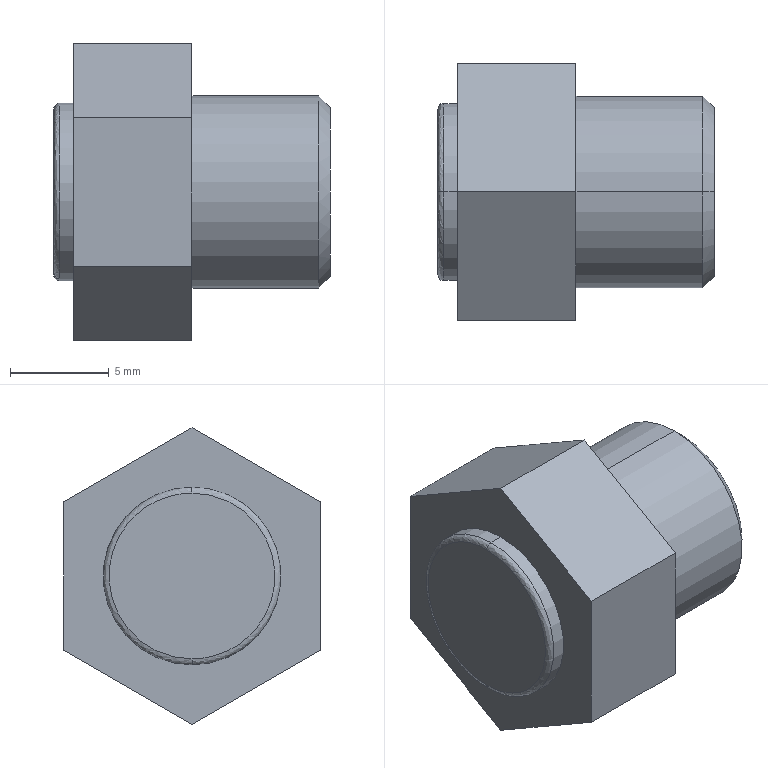Part | STEP file | GRM4_BREATHER_VENT_71996_M | 1 solid | 18 faces | box 14 x 13 x 15.011 mm | volume 1457 mm3 | plane 10 | cylinder 4 | spline 2 | cone 2 | commonest cylinder face diameters 9 x2 9.728 x2
STEP:
#1=CARTESIAN_POINT('',(-6.7,0.,4.5));
#2=VERTEX_POINT('',#1);
#3=CARTESIAN_POINT('',(-6.7,0.,-4.5));
#4=VERTEX_POINT('',#3);
#5=CARTESIAN_POINT('',(-6.7,0.,0.));
#6=DIRECTION('',(1.,0.,0.));
#7=DIRECTION('',(0.,0.,-1.));
#8=AXIS2_PLACEMENT_3D('',#5,#6,#7);
#9=CIRCLE('',#8,4.5);
#10=EDGE_CURVE('',#2,#4,#9,.T.);
#11=ORIENTED_EDGE('',*,*,#10,.F.);
#12=CARTESIAN_POINT('',(-7.,0.,4.2));
#13=VERTEX_POINT('',#12);
#14=CARTESIAN_POINT('',(-6.7,0.,4.2));
#15=DIRECTION('',(0.,-1.,0.));
#16=DIRECTION('',(0.,0.,1.));
#17=AXIS2_PLACEMENT_3D('',#14,#15,#16);
#18=CIRCLE('',#17,0.3);
#19=EDGE_CURVE('',#2,#13,#18,.T.);
#20=ORIENTED_EDGE('',*,*,#19,.T.);
#21=CARTESIAN_POINT('',(-7.,0.,-4.2));
#22=VERTEX_POINT('',#21);
#23=CARTESIAN_POINT('',(-7.,0.,4.2));
#24=CARTESIAN_POINT('',(-7.,-8.4,4.2));
#25=CARTESIAN_POINT('',(-7.,-8.4,-4.2));
#26=CARTESIAN_POINT('',(-7.,0.,-4.2));
#27=(BOUNDED_CURVE()B_SPLINE_CURVE(3,(#23,#24,#25,#26),.UNSPECIFIED.,.F.,.T.)B_SPLINE_CURVE_WITH_KNOTS((4,4),(0.5,1.),.UNSPECIFIED.)CURVE()GEOMETRIC_REPRESENTATION_ITEM()RATIONAL_B_SPLINE_CURVE((1.,0.3333,0.3333,1.))REPRESENTATION_ITEM(''));
#28=EDGE_CURVE('',#13,#22,#27,.T.);
#29=ORIENTED_EDGE('',*,*,#28,.T.);
#30=CARTESIAN_POINT('',(-6.7,0.,-4.2));
#31=DIRECTION('',(0.,1.,0.));
#32=DIRECTION('',(0.,0.,-1.));
#33=AXIS2_PLACEMENT_3D('',#30,#31,#32);
#34=CIRCLE('',#33,0.3);
#35=EDGE_CURVE('',#4,#22,#34,.T.);
#36=ORIENTED_EDGE('',*,*,#35,.F.);
#37=EDGE_LOOP('',(#11,#20,#29,#36));
#38=FACE_OUTER_BOUND('',#37,.T.);
#39=CARTESIAN_POINT('',(-6.7,0.,4.5));
#40=CARTESIAN_POINT('',(-6.7,-9.,4.5));
#41=CARTESIAN_POINT('',(-6.7,-9.,-4.5));
#42=CARTESIAN_POINT('',(-6.7,0.,-4.5));
#43=CARTESIAN_POINT('',(-6.876,0.,4.5));
#44=CARTESIAN_POINT('',(-6.876,-9.,4.5));
#45=CARTESIAN_POINT('',(-6.876,-9.,-4.5));
#46=CARTESIAN_POINT('',(-6.876,0.,-4.5));
#47=CARTESIAN_POINT('',(-7.,0.,4.376));
#48=CARTESIAN_POINT('',(-7.,-8.751,4.376));
#49=CARTESIAN_POINT('',(-7.,-8.751,-4.376));
#50=CARTESIAN_POINT('',(-7.,0.,-4.376));
#51=CARTESIAN_POINT('',(-7.,0.,4.2));
#52=CARTESIAN_POINT('',(-7.,-8.4,4.2));
#53=CARTESIAN_POINT('',(-7.,-8.4,-4.2));
#54=CARTESIAN_POINT('',(-7.,0.,-4.2));
#55=(BOUNDED_SURFACE()B_SPLINE_SURFACE(3,3,((#39,#40,#41,#42),(#43,#44,#45,#46),(#47,#48,#49,#50),(#51,#52,#53,#54)),.UNSPECIFIED.,.F.,.F.,.F.)B_SPLINE_SURFACE_WITH_KNOTS((4,4),(4,4),(0.,1.),(0.,1.),.UNSPECIFIED.)GEOMETRIC_REPRESENTATION_ITEM()RATIONAL_B_SPLINE_SURFACE(((1.,0.3333,0.3333,1.),(0.8047,0.2682,0.2682,0.8047),(0.8047,0.2682,0.2682,0.8047),(1.,0.3333,0.3333,1.)))REPRESENTATION_ITEM('')SURFACE());
#56=ADVANCED_FACE('',(#38),#55,.T.);
#57=CARTESIAN_POINT('',(0.,0.,-4.864));
#58=VERTEX_POINT('',#57);
#59=CARTESIAN_POINT('',(0.,0.,4.864));
#60=VERTEX_POINT('',#59);
#61=CARTESIAN_POINT('',(0.,0.,0.));
#62=DIRECTION('',(1.,0.,0.));
#63=DIRECTION('',(0.,0.,-1.));
#64=AXIS2_PLACEMENT_3D('',#61,#62,#63);
#65=CIRCLE('',#64,4.864);
#66=EDGE_CURVE('',#58,#60,#65,.T.);
#67=ORIENTED_EDGE('',*,*,#66,.T.);
#68=CARTESIAN_POINT('',(6.419,0.,4.864));
#69=VERTEX_POINT('',#68);
#70=CARTESIAN_POINT('',(7.,0.,4.864));
#71=DIRECTION('',(1.,0.,0.));
#72=VECTOR('',#71,1000.);
#73=LINE('',#70,#72);
#74=EDGE_CURVE('',#60,#69,#73,.T.);
#75=ORIENTED_EDGE('',*,*,#74,.T.);
#76=CARTESIAN_POINT('',(6.419,0.,-4.864));
#77=VERTEX_POINT('',#76);
#78=CARTESIAN_POINT('',(6.419,0.,0.));
#79=DIRECTION('',(-1.,0.,0.));
#80=DIRECTION('',(0.,0.,-1.));
#81=AXIS2_PLACEMENT_3D('',#78,#79,#80);
#82=CIRCLE('',#81,4.864);
#83=EDGE_CURVE('',#69,#77,#82,.T.);
#84=ORIENTED_EDGE('',*,*,#83,.T.);
#85=CARTESIAN_POINT('',(7.,0.,-4.864));
#86=DIRECTION('',(1.,0.,0.));
#87=VECTOR('',#86,1000.);
#88=LINE('',#85,#87);
#89=EDGE_CURVE('',#58,#77,#88,.T.);
#90=ORIENTED_EDGE('',*,*,#89,.F.);
#91=EDGE_LOOP('',(#67,#75,#84,#90));
#92=FACE_OUTER_BOUND('',#91,.T.);
#93=CARTESIAN_POINT('',(7.,0.,0.));
#94=DIRECTION('',(1.,0.,0.));
#95=DIRECTION('',(0.,0.,-1.));
#96=AXIS2_PLACEMENT_3D('',#93,#94,#95);
#97=CYLINDRICAL_SURFACE('',#96,4.864);
#98=ADVANCED_FACE('',(#92),#97,.T.);
#99=CARTESIAN_POINT('',(7.,0.,4.283));
#100=VERTEX_POINT('',#99);
#101=CARTESIAN_POINT('',(7.,0.,-4.283));
#102=VERTEX_POINT('',#101);
#103=CARTESIAN_POINT('',(7.,0.,0.));
#104=DIRECTION('',(-1.,0.,0.));
#105=DIRECTION('',(0.,0.,1.));
#106=AXIS2_PLACEMENT_3D('',#103,#104,#105);
#107=CIRCLE('',#106,4.283);
#108=EDGE_CURVE('',#100,#102,#107,.T.);
#109=ORIENTED_EDGE('',*,*,#108,.T.);
#110=CARTESIAN_POINT('',(6.419,0.,-4.864));
#111=DIRECTION('',(-0.7071,0.,-0.7071));
#112=VECTOR('',#111,1000.);
#113=LINE('',#110,#112);
#114=EDGE_CURVE('',#102,#77,#113,.T.);
#115=ORIENTED_EDGE('',*,*,#114,.T.);
#116=ORIENTED_EDGE('',*,*,#83,.F.);
#117=CARTESIAN_POINT('',(6.419,0.,4.864));
#118=DIRECTION('',(-0.7071,0.,0.7071));
#119=VECTOR('',#118,1000.);
#120=LINE('',#117,#119);
#121=EDGE_CURVE('',#100,#69,#120,.T.);
#122=ORIENTED_EDGE('',*,*,#121,.F.);
#123=EDGE_LOOP('',(#109,#115,#116,#122));
#124=FACE_OUTER_BOUND('',#123,.T.);
#125=CARTESIAN_POINT('',(6.419,0.,0.));
#126=DIRECTION('',(-1.,0.,0.));
#127=DIRECTION('',(0.,0.,1.));
#128=AXIS2_PLACEMENT_3D('',#125,#126,#127);
#129=CONICAL_SURFACE('',#128,4.864,0.7854);
#130=ADVANCED_FACE('',(#124),#129,.T.);
#131=CARTESIAN_POINT('',(-6.7,0.,0.));
#132=DIRECTION('',(1.,0.,0.));
#133=DIRECTION('',(0.,0.,-1.));
#134=AXIS2_PLACEMENT_3D('',#131,#132,#133);
#135=CIRCLE('',#134,4.5);
#136=EDGE_CURVE('',#4,#2,#135,.T.);
#137=ORIENTED_EDGE('',*,*,#136,.T.);
#138=CARTESIAN_POINT('',(-6.,0.,4.5));
#139=VERTEX_POINT('',#138);
#140=CARTESIAN_POINT('',(7.,0.,4.5));
#141=DIRECTION('',(1.,0.,0.));
#142=VECTOR('',#141,1000.);
#143=LINE('',#140,#142);
#144=EDGE_CURVE('',#2,#139,#143,.T.);
#145=ORIENTED_EDGE('',*,*,#144,.T.);
#146=CARTESIAN_POINT('',(-6.,0.,-4.5));
#147=VERTEX_POINT('',#146);
#148=CARTESIAN_POINT('',(-6.,0.,0.));
#149=DIRECTION('',(1.,0.,0.));
#150=DIRECTION('',(0.,0.,-1.));
#151=AXIS2_PLACEMENT_3D('',#148,#149,#150);
#152=CIRCLE('',#151,4.5);
#153=EDGE_CURVE('',#147,#139,#152,.T.);
#154=ORIENTED_EDGE('',*,*,#153,.F.);
#155=CARTESIAN_POINT('',(7.,0.,-4.5));
#156=DIRECTION('',(1.,0.,0.));
#157=VECTOR('',#156,1000.);
#158=LINE('',#155,#157);
#159=EDGE_CURVE('',#4,#147,#158,.T.);
#160=ORIENTED_EDGE('',*,*,#159,.F.);
#161=EDGE_LOOP('',(#137,#145,#154,#160));
#162=FACE_OUTER_BOUND('',#161,.T.);
#163=CARTESIAN_POINT('',(7.,0.,0.));
#164=DIRECTION('',(1.,0.,0.));
#165=DIRECTION('',(0.,0.,-1.));
#166=AXIS2_PLACEMENT_3D('',#163,#164,#165);
#167=CYLINDRICAL_SURFACE('',#166,4.5);
#168=ADVANCED_FACE('',(#162),#167,.T.);
#169=ORIENTED_EDGE('',*,*,#74,.F.);
#170=CARTESIAN_POINT('',(0.,0.,0.));
#171=DIRECTION('',(1.,0.,0.));
#172=DIRECTION('',(0.,0.,-1.));
#173=AXIS2_PLACEMENT_3D('',#170,#171,#172);
#174=CIRCLE('',#173,4.864);
#175=EDGE_CURVE('',#60,#58,#174,.T.);
#176=ORIENTED_EDGE('',*,*,#175,.T.);
#177=ORIENTED_EDGE('',*,*,#89,.T.);
#178=CARTESIAN_POINT('',(6.419,0.,0.));
#179=DIRECTION('',(-1.,0.,0.));
#180=DIRECTION('',(0.,0.,-1.));
#181=AXIS2_PLACEMENT_3D('',#178,#179,#180);
#182=CIRCLE('',#181,4.864);
#183=EDGE_CURVE('',#77,#69,#182,.T.);
#184=ORIENTED_EDGE('',*,*,#183,.T.);
#185=EDGE_LOOP('',(#169,#176,#177,#184));
#186=FACE_OUTER_BOUND('',#185,.T.);
#187=CARTESIAN_POINT('',(7.,0.,0.));
#188=DIRECTION('',(1.,0.,0.));
#189=DIRECTION('',(0.,0.,-1.));
#190=AXIS2_PLACEMENT_3D('',#187,#188,#189);
#191=CYLINDRICAL_SURFACE('',#190,4.864);
#192=ADVANCED_FACE('',(#186),#191,.T.);
#193=CARTESIAN_POINT('',(0.,0.,-7.506));
#194=VERTEX_POINT('',#193);
#195=CARTESIAN_POINT('',(0.,-6.5,-3.753));
#196=VERTEX_POINT('',#195);
#197=CARTESIAN_POINT('',(0.,0.,-7.506));
#198=DIRECTION('',(0.,-0.866,0.5));
#199=VECTOR('',#198,1000.);
#200=LINE('',#197,#199);
#201=EDGE_CURVE('',#194,#196,#200,.T.);
#202=ORIENTED_EDGE('',*,*,#201,.F.);
#203=CARTESIAN_POINT('',(0.,6.5,-3.753));
#204=VERTEX_POINT('',#203);
#205=CARTESIAN_POINT('',(0.,6.5,-3.753));
#206=DIRECTION('',(0.,-0.866,-0.5));
#207=VECTOR('',#206,1000.);
#208=LINE('',#205,#207);
#209=EDGE_CURVE('',#204,#194,#208,.T.);
#210=ORIENTED_EDGE('',*,*,#209,.F.);
#211=CARTESIAN_POINT('',(0.,6.5,3.753));
#212=VERTEX_POINT('',#211);
#213=CARTESIAN_POINT('',(0.,6.5,0.));
#214=DIRECTION('',(0.,0.,-1.));
#215=VECTOR('',#214,1000.);
#216=LINE('',#213,#215);
#217=EDGE_CURVE('',#212,#204,#216,.T.);
#218=ORIENTED_EDGE('',*,*,#217,.F.);
#219=CARTESIAN_POINT('',(0.,0.,7.506));
#220=VERTEX_POINT('',#219);
#221=CARTESIAN_POINT('',(0.,0.,7.506));
#222=DIRECTION('',(0.,0.866,-0.5));
#223=VECTOR('',#222,1000.);
#224=LINE('',#221,#223);
#225=EDGE_CURVE('',#220,#212,#224,.T.);
#226=ORIENTED_EDGE('',*,*,#225,.F.);
#227=CARTESIAN_POINT('',(0.,-6.5,3.753));
#228=VERTEX_POINT('',#227);
#229=CARTESIAN_POINT('',(0.,-6.5,3.753));
#230=DIRECTION('',(0.,0.866,0.5));
#231=VECTOR('',#230,1000.);
#232=LINE('',#229,#231);
#233=EDGE_CURVE('',#228,#220,#232,.T.);
#234=ORIENTED_EDGE('',*,*,#233,.F.);
#235=CARTESIAN_POINT('',(0.,-6.5,0.));
#236=DIRECTION('',(0.,0.,1.));
#237=VECTOR('',#236,1000.);
#238=LINE('',#235,#237);
#239=EDGE_CURVE('',#196,#228,#238,.T.);
#240=ORIENTED_EDGE('',*,*,#239,.F.);
#241=EDGE_LOOP('',(#202,#210,#218,#226,#234,#240));
#242=FACE_OUTER_BOUND('',#241,.T.);
#243=ORIENTED_EDGE('',*,*,#66,.F.);
#244=ORIENTED_EDGE('',*,*,#175,.F.);
#245=EDGE_LOOP('',(#243,#244));
#246=FACE_BOUND('',#245,.T.);
#247=CARTESIAN_POINT('',(0.,0.,0.));
#248=DIRECTION('',(-1.,0.,0.));
#249=DIRECTION('',(0.,0.,1.));
#250=AXIS2_PLACEMENT_3D('',#247,#248,#249);
#251=PLANE('',#250);
#252=ADVANCED_FACE('',(#242,#246),#251,.F.);
#253=ORIENTED_EDGE('',*,*,#114,.F.);
#254=CARTESIAN_POINT('',(7.,0.,0.));
#255=DIRECTION('',(-1.,0.,0.));
#256=DIRECTION('',(0.,0.,1.));
#257=AXIS2_PLACEMENT_3D('',#254,#255,#256);
#258=CIRCLE('',#257,4.283);
#259=EDGE_CURVE('',#102,#100,#258,.T.);
#260=ORIENTED_EDGE('',*,*,#259,.T.);
#261=ORIENTED_EDGE('',*,*,#121,.T.);
#262=ORIENTED_EDGE('',*,*,#183,.F.);
#263=EDGE_LOOP('',(#253,#260,#261,#262));
#264=FACE_OUTER_BOUND('',#263,.T.);
#265=CARTESIAN_POINT('',(6.419,0.,0.));
#266=DIRECTION('',(-1.,0.,0.));
#267=DIRECTION('',(0.,0.,1.));
#268=AXIS2_PLACEMENT_3D('',#265,#266,#267);
#269=CONICAL_SURFACE('',#268,4.864,0.7854);
#270=ADVANCED_FACE('',(#264),#269,.T.);
#271=CARTESIAN_POINT('',(-6.,-6.5,3.753));
#272=VERTEX_POINT('',#271);
#273=CARTESIAN_POINT('',(-6.,-6.5,3.753));
#274=DIRECTION('',(1.,0.,0.));
#275=VECTOR('',#274,1000.);
#276=LINE('',#273,#275);
#277=EDGE_CURVE('',#272,#228,#276,.T.);
#278=ORIENTED_EDGE('',*,*,#277,.F.);
#279=CARTESIAN_POINT('',(-6.,-6.5,-3.753));
#280=VERTEX_POINT('',#279);
#281=CARTESIAN_POINT('',(-6.,-6.5,-3.753));
#282=DIRECTION('',(0.,0.,1.));
#283=VECTOR('',#282,1000.);
#284=LINE('',#281,#283);
#285=EDGE_CURVE('',#280,#272,#284,.T.);
#286=ORIENTED_EDGE('',*,*,#285,.F.);
#287=CARTESIAN_POINT('',(-6.,-6.5,-3.753));
#288=DIRECTION('',(-1.,0.,0.));
#289=VECTOR('',#288,1000.);
#290=LINE('',#287,#289);
#291=EDGE_CURVE('',#196,#280,#290,.T.);
#292=ORIENTED_EDGE('',*,*,#291,.F.);
#293=ORIENTED_EDGE('',*,*,#239,.T.);
#294=EDGE_LOOP('',(#278,#286,#292,#293));
#295=FACE_OUTER_BOUND('',#294,.T.);
#296=CARTESIAN_POINT('',(-6.,-6.5,-3.753));
#297=DIRECTION('',(0.,1.,0.));
#298=DIRECTION('',(0.,0.,1.));
#299=AXIS2_PLACEMENT_3D('',#296,#297,#298);
#300=PLANE('',#299);
#301=ADVANCED_FACE('',(#295),#300,.F.);
#302=ORIENTED_EDGE('',*,*,#291,.T.);
#303=CARTESIAN_POINT('',(-6.,0.,-7.506));
#304=VERTEX_POINT('',#303);
#305=CARTESIAN_POINT('',(-6.,0.,-7.506));
#306=DIRECTION('',(0.,-0.866,0.5));
#307=VECTOR('',#306,1000.);
#308=LINE('',#305,#307);
#309=EDGE_CURVE('',#304,#280,#308,.T.);
#310=ORIENTED_EDGE('',*,*,#309,.F.);
#311=CARTESIAN_POINT('',(-6.,0.,-7.506));
#312=DIRECTION('',(-1.,0.,0.));
#313=VECTOR('',#312,1000.);
#314=LINE('',#311,#313);
#315=EDGE_CURVE('',#194,#304,#314,.T.);
#316=ORIENTED_EDGE('',*,*,#315,.F.);
#317=ORIENTED_EDGE('',*,*,#201,.T.);
#318=EDGE_LOOP('',(#302,#310,#316,#317));
#319=FACE_OUTER_BOUND('',#318,.T.);
#320=CARTESIAN_POINT('',(-6.,0.,-7.506));
#321=DIRECTION('',(0.,0.5,0.866));
#322=DIRECTION('',(0.,-0.866,0.5));
#323=AXIS2_PLACEMENT_3D('',#320,#321,#322);
#324=PLANE('',#323);
#325=ADVANCED_FACE('',(#319),#324,.F.);
#326=ORIENTED_EDGE('',*,*,#315,.T.);
#327=CARTESIAN_POINT('',(-6.,6.5,-3.753));
#328=VERTEX_POINT('',#327);
#329=CARTESIAN_POINT('',(-6.,6.5,-3.753));
#330=DIRECTION('',(0.,-0.866,-0.5));
#331=VECTOR('',#330,1000.);
#332=LINE('',#329,#331);
#333=EDGE_CURVE('',#328,#304,#332,.T.);
#334=ORIENTED_EDGE('',*,*,#333,.F.);
#335=CARTESIAN_POINT('',(-6.,6.5,-3.753));
#336=DIRECTION('',(-1.,0.,0.));
#337=VECTOR('',#336,1000.);
#338=LINE('',#335,#337);
#339=EDGE_CURVE('',#204,#328,#338,.T.);
#340=ORIENTED_EDGE('',*,*,#339,.F.);
#341=ORIENTED_EDGE('',*,*,#209,.T.);
#342=EDGE_LOOP('',(#326,#334,#340,#341));
#343=FACE_OUTER_BOUND('',#342,.T.);
#344=CARTESIAN_POINT('',(-6.,6.5,-3.753));
#345=DIRECTION('',(0.,-0.5,0.866));
#346=DIRECTION('',(0.,-0.866,-0.5));
#347=AXIS2_PLACEMENT_3D('',#344,#345,#346);
#348=PLANE('',#347);
#349=ADVANCED_FACE('',(#343),#348,.F.);
#350=ORIENTED_EDGE('',*,*,#339,.T.);
#351=CARTESIAN_POINT('',(-6.,6.5,3.753));
#352=VERTEX_POINT('',#351);
#353=CARTESIAN_POINT('',(-6.,6.5,3.753));
#354=DIRECTION('',(0.,0.,-1.));
#355=VECTOR('',#354,1000.);
#356=LINE('',#353,#355);
#357=EDGE_CURVE('',#352,#328,#356,.T.);
#358=ORIENTED_EDGE('',*,*,#357,.F.);
#359=CARTESIAN_POINT('',(-6.,6.5,3.753));
#360=DIRECTION('',(-1.,0.,0.));
#361=VECTOR('',#360,1000.);
#362=LINE('',#359,#361);
#363=EDGE_CURVE('',#212,#352,#362,.T.);
#364=ORIENTED_EDGE('',*,*,#363,.F.);
#365=ORIENTED_EDGE('',*,*,#217,.T.);
#366=EDGE_LOOP('',(#350,#358,#364,#365));
#367=FACE_OUTER_BOUND('',#366,.T.);
#368=CARTESIAN_POINT('',(-6.,6.5,3.753));
#369=DIRECTION('',(0.,-1.,0.));
#370=DIRECTION('',(0.,0.,-1.));
#371=AXIS2_PLACEMENT_3D('',#368,#369,#370);
#372=PLANE('',#371);
#373=ADVANCED_FACE('',(#367),#372,.F.);
#374=ORIENTED_EDGE('',*,*,#363,.T.);
#375=CARTESIAN_POINT('',(-6.,0.,7.506));
#376=VERTEX_POINT('',#375);
#377=CARTESIAN_POINT('',(-6.,0.,7.506));
#378=DIRECTION('',(0.,0.866,-0.5));
#379=VECTOR('',#378,1000.);
#380=LINE('',#377,#379);
#381=EDGE_CURVE('',#376,#352,#380,.T.);
#382=ORIENTED_EDGE('',*,*,#381,.F.);
#383=CARTESIAN_POINT('',(-6.,0.,7.506));
#384=DIRECTION('',(-1.,0.,0.));
#385=VECTOR('',#384,1000.);
#386=LINE('',#383,#385);
#387=EDGE_CURVE('',#220,#376,#386,.T.);
#388=ORIENTED_EDGE('',*,*,#387,.F.);
#389=ORIENTED_EDGE('',*,*,#225,.T.);
#390=EDGE_LOOP('',(#374,#382,#388,#389));
#391=FACE_OUTER_BOUND('',#390,.T.);
#392=CARTESIAN_POINT('',(-6.,0.,7.506));
#393=DIRECTION('',(0.,-0.5,-0.866));
#394=DIRECTION('',(0.,0.866,-0.5));
#395=AXIS2_PLACEMENT_3D('',#392,#393,#394);
#396=PLANE('',#395);
#397=ADVANCED_FACE('',(#391),#396,.F.);
#398=ORIENTED_EDGE('',*,*,#387,.T.);
#399=CARTESIAN_POINT('',(-6.,-6.5,3.753));
#400=DIRECTION('',(0.,0.866,0.5));
#401=VECTOR('',#400,1000.);
#402=LINE('',#399,#401);
#403=EDGE_CURVE('',#272,#376,#402,.T.);
#404=ORIENTED_EDGE('',*,*,#403,.F.);
#405=ORIENTED_EDGE('',*,*,#277,.T.);
#406=ORIENTED_EDGE('',*,*,#233,.T.);
#407=EDGE_LOOP('',(#398,#404,#405,#406));
#408=FACE_OUTER_BOUND('',#407,.T.);
#409=CARTESIAN_POINT('',(-6.,-6.5,3.753));
#410=DIRECTION('',(0.,0.5,-0.866));
#411=DIRECTION('',(0.,0.866,0.5));
#412=AXIS2_PLACEMENT_3D('',#409,#410,#411);
#413=PLANE('',#412);
#414=ADVANCED_FACE('',(#408),#413,.F.);
#415=ORIENTED_EDGE('',*,*,#108,.F.);
#416=ORIENTED_EDGE('',*,*,#259,.F.);
#417=EDGE_LOOP('',(#415,#416));
#418=FACE_OUTER_BOUND('',#417,.T.);
#419=CARTESIAN_POINT('',(7.,4.283,0.));
#420=DIRECTION('',(-1.,0.,0.));
#421=DIRECTION('',(0.,0.,1.));
#422=AXIS2_PLACEMENT_3D('',#419,#420,#421);
#423=PLANE('',#422);
#424=ADVANCED_FACE('',(#418),#423,.F.);
#425=ORIENTED_EDGE('',*,*,#333,.T.);
#426=ORIENTED_EDGE('',*,*,#309,.T.);
#427=ORIENTED_EDGE('',*,*,#285,.T.);
#428=ORIENTED_EDGE('',*,*,#403,.T.);
#429=ORIENTED_EDGE('',*,*,#381,.T.);
#430=ORIENTED_EDGE('',*,*,#357,.T.);
#431=EDGE_LOOP('',(#425,#426,#427,#428,#429,#430));
#432=FACE_OUTER_BOUND('',#431,.T.);
#433=ORIENTED_EDGE('',*,*,#153,.T.);
#434=CARTESIAN_POINT('',(-6.,0.,0.));
#435=DIRECTION('',(1.,0.,0.));
#436=DIRECTION('',(0.,0.,-1.));
#437=AXIS2_PLACEMENT_3D('',#434,#435,#436);
#438=CIRCLE('',#437,4.5);
#439=EDGE_CURVE('',#139,#147,#438,.T.);
#440=ORIENTED_EDGE('',*,*,#439,.T.);
#441=EDGE_LOOP('',(#433,#440));
#442=FACE_BOUND('',#441,.T.);
#443=CARTESIAN_POINT('',(-6.,0.,0.));
#444=DIRECTION('',(-1.,0.,0.));
#445=DIRECTION('',(0.,0.,1.));
#446=AXIS2_PLACEMENT_3D('',#443,#444,#445);
#447=PLANE('',#446);
#448=ADVANCED_FACE('',(#432,#442),#447,.T.);
#449=ORIENTED_EDGE('',*,*,#144,.F.);
#450=ORIENTED_EDGE('',*,*,#10,.T.);
#451=ORIENTED_EDGE('',*,*,#159,.T.);
#452=ORIENTED_EDGE('',*,*,#439,.F.);
#453=EDGE_LOOP('',(#449,#450,#451,#452));
#454=FACE_OUTER_BOUND('',#453,.T.);
#455=CARTESIAN_POINT('',(7.,0.,0.));
#456=DIRECTION('',(1.,0.,0.));
#457=DIRECTION('',(0.,0.,-1.));
#458=AXIS2_PLACEMENT_3D('',#455,#456,#457);
#459=CYLINDRICAL_SURFACE('',#458,4.5);
#460=ADVANCED_FACE('',(#454),#459,.T.);
#461=ORIENTED_EDGE('',*,*,#19,.F.);
#462=ORIENTED_EDGE('',*,*,#136,.F.);
#463=ORIENTED_EDGE('',*,*,#35,.T.);
#464=CARTESIAN_POINT('',(-7.,0.,-4.2));
#465=CARTESIAN_POINT('',(-7.,8.4,-4.2));
#466=CARTESIAN_POINT('',(-7.,8.4,4.2));
#467=CARTESIAN_POINT('',(-7.,0.,4.2));
#468=(BOUNDED_CURVE()B_SPLINE_CURVE(3,(#464,#465,#466,#467),.UNSPECIFIED.,.F.,.F.)B_SPLINE_CURVE_WITH_KNOTS((4,4),(0.,0.5),.UNSPECIFIED.)CURVE()GEOMETRIC_REPRESENTATION_ITEM()RATIONAL_B_SPLINE_CURVE((1.,0.3333,0.3333,1.))REPRESENTATION_ITEM(''));
#469=EDGE_CURVE('',#22,#13,#468,.T.);
#470=ORIENTED_EDGE('',*,*,#469,.T.);
#471=EDGE_LOOP('',(#461,#462,#463,#470));
#472=FACE_OUTER_BOUND('',#471,.T.);
#473=CARTESIAN_POINT('',(-6.7,0.,-4.5));
#474=CARTESIAN_POINT('',(-6.7,9.,-4.5));
#475=CARTESIAN_POINT('',(-6.7,9.,4.5));
#476=CARTESIAN_POINT('',(-6.7,0.,4.5));
#477=CARTESIAN_POINT('',(-6.876,0.,-4.5));
#478=CARTESIAN_POINT('',(-6.876,9.,-4.5));
#479=CARTESIAN_POINT('',(-6.876,9.,4.5));
#480=CARTESIAN_POINT('',(-6.876,0.,4.5));
#481=CARTESIAN_POINT('',(-7.,0.,-4.376));
#482=CARTESIAN_POINT('',(-7.,8.751,-4.376));
#483=CARTESIAN_POINT('',(-7.,8.751,4.376));
#484=CARTESIAN_POINT('',(-7.,0.,4.376));
#485=CARTESIAN_POINT('',(-7.,0.,-4.2));
#486=CARTESIAN_POINT('',(-7.,8.4,-4.2));
#487=CARTESIAN_POINT('',(-7.,8.4,4.2));
#488=CARTESIAN_POINT('',(-7.,0.,4.2));
#489=(BOUNDED_SURFACE()B_SPLINE_SURFACE(3,3,((#473,#474,#475,#476),(#477,#478,#479,#480),(#481,#482,#483,#484),(#485,#486,#487,#488)),.UNSPECIFIED.,.F.,.F.,.F.)B_SPLINE_SURFACE_WITH_KNOTS((4,4),(4,4),(0.,1.),(0.,1.),.UNSPECIFIED.)GEOMETRIC_REPRESENTATION_ITEM()RATIONAL_B_SPLINE_SURFACE(((1.,0.3333,0.3333,1.),(0.8047,0.2682,0.2682,0.8047),(0.8047,0.2682,0.2682,0.8047),(1.,0.3333,0.3333,1.)))REPRESENTATION_ITEM('')SURFACE());
#490=ADVANCED_FACE('',(#472),#489,.T.);
#491=ORIENTED_EDGE('',*,*,#469,.F.);
#492=ORIENTED_EDGE('',*,*,#28,.F.);
#493=EDGE_LOOP('',(#491,#492));
#494=FACE_OUTER_BOUND('',#493,.T.);
#495=CARTESIAN_POINT('',(-7.,0.,0.));
#496=DIRECTION('',(1.,0.,0.));
#497=DIRECTION('',(0.,0.,-1.));
#498=AXIS2_PLACEMENT_3D('',#495,#496,#497);
#499=PLANE('',#498);
#500=ADVANCED_FACE('',(#494),#499,.F.);
#501=CLOSED_SHELL('',(#56,#98,#130,#168,#192,#252,#270,#301,#325,#349,#373,#397,#414,#424,#448,#460,#490,#500));
#502=MANIFOLD_SOLID_BREP('',#501);
#503=CARTESIAN_POINT('',(0.,0.,0.));
#504=DIRECTION('',(0.,0.,1.));
#505=DIRECTION('',(1.,0.,0.));
#506=AXIS2_PLACEMENT_3D('',#503,#504,#505);
#507=(LENGTH_UNIT()NAMED_UNIT(*)SI_UNIT(.MILLI.,.METRE.));
#508=UNCERTAINTY_MEASURE_WITH_UNIT(LENGTH_MEASURE(0.00001),#507,'','');
#509=(NAMED_UNIT(*)PLANE_ANGLE_UNIT()SI_UNIT($,.RADIAN.));
#510=(NAMED_UNIT(*)SI_UNIT($,.STERADIAN.)SOLID_ANGLE_UNIT());
#511=(GEOMETRIC_REPRESENTATION_CONTEXT(3)GLOBAL_UNCERTAINTY_ASSIGNED_CONTEXT((#508))GLOBAL_UNIT_ASSIGNED_CONTEXT((#507,#509,#510))REPRESENTATION_CONTEXT('',''));
#512=ADVANCED_BREP_SHAPE_REPRESENTATION('',(#502,#506),#511);